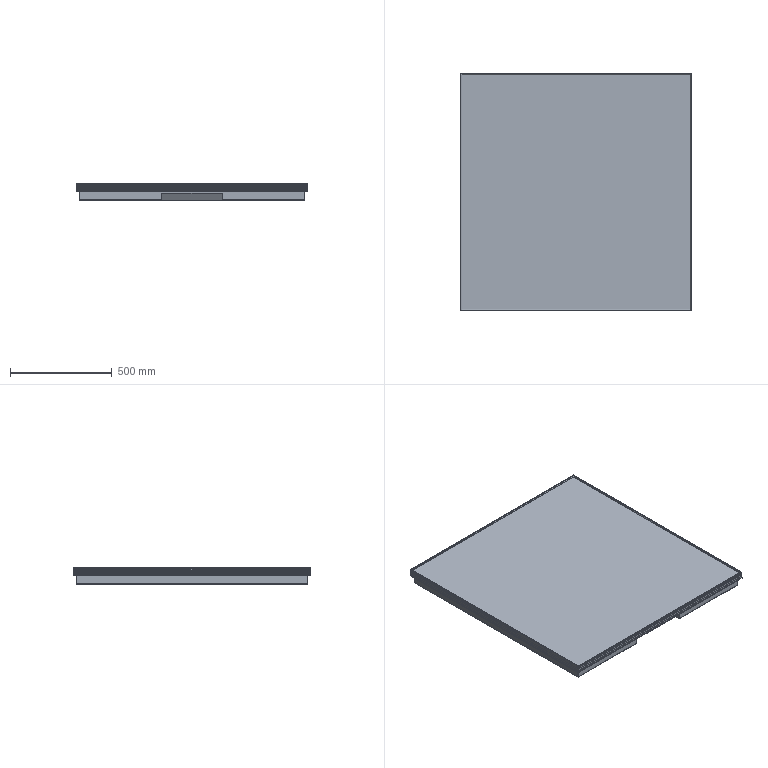Part | 8 solids | 408 faces | box 1140 x 1170 x 80 mm | volume 7247034 mm3 | plane 254 | cylinder 142 | spline 12 | commonest cylinder face diameters 7 x100 14 x14 1 x9 3 x9 5 x4 0.4 x2